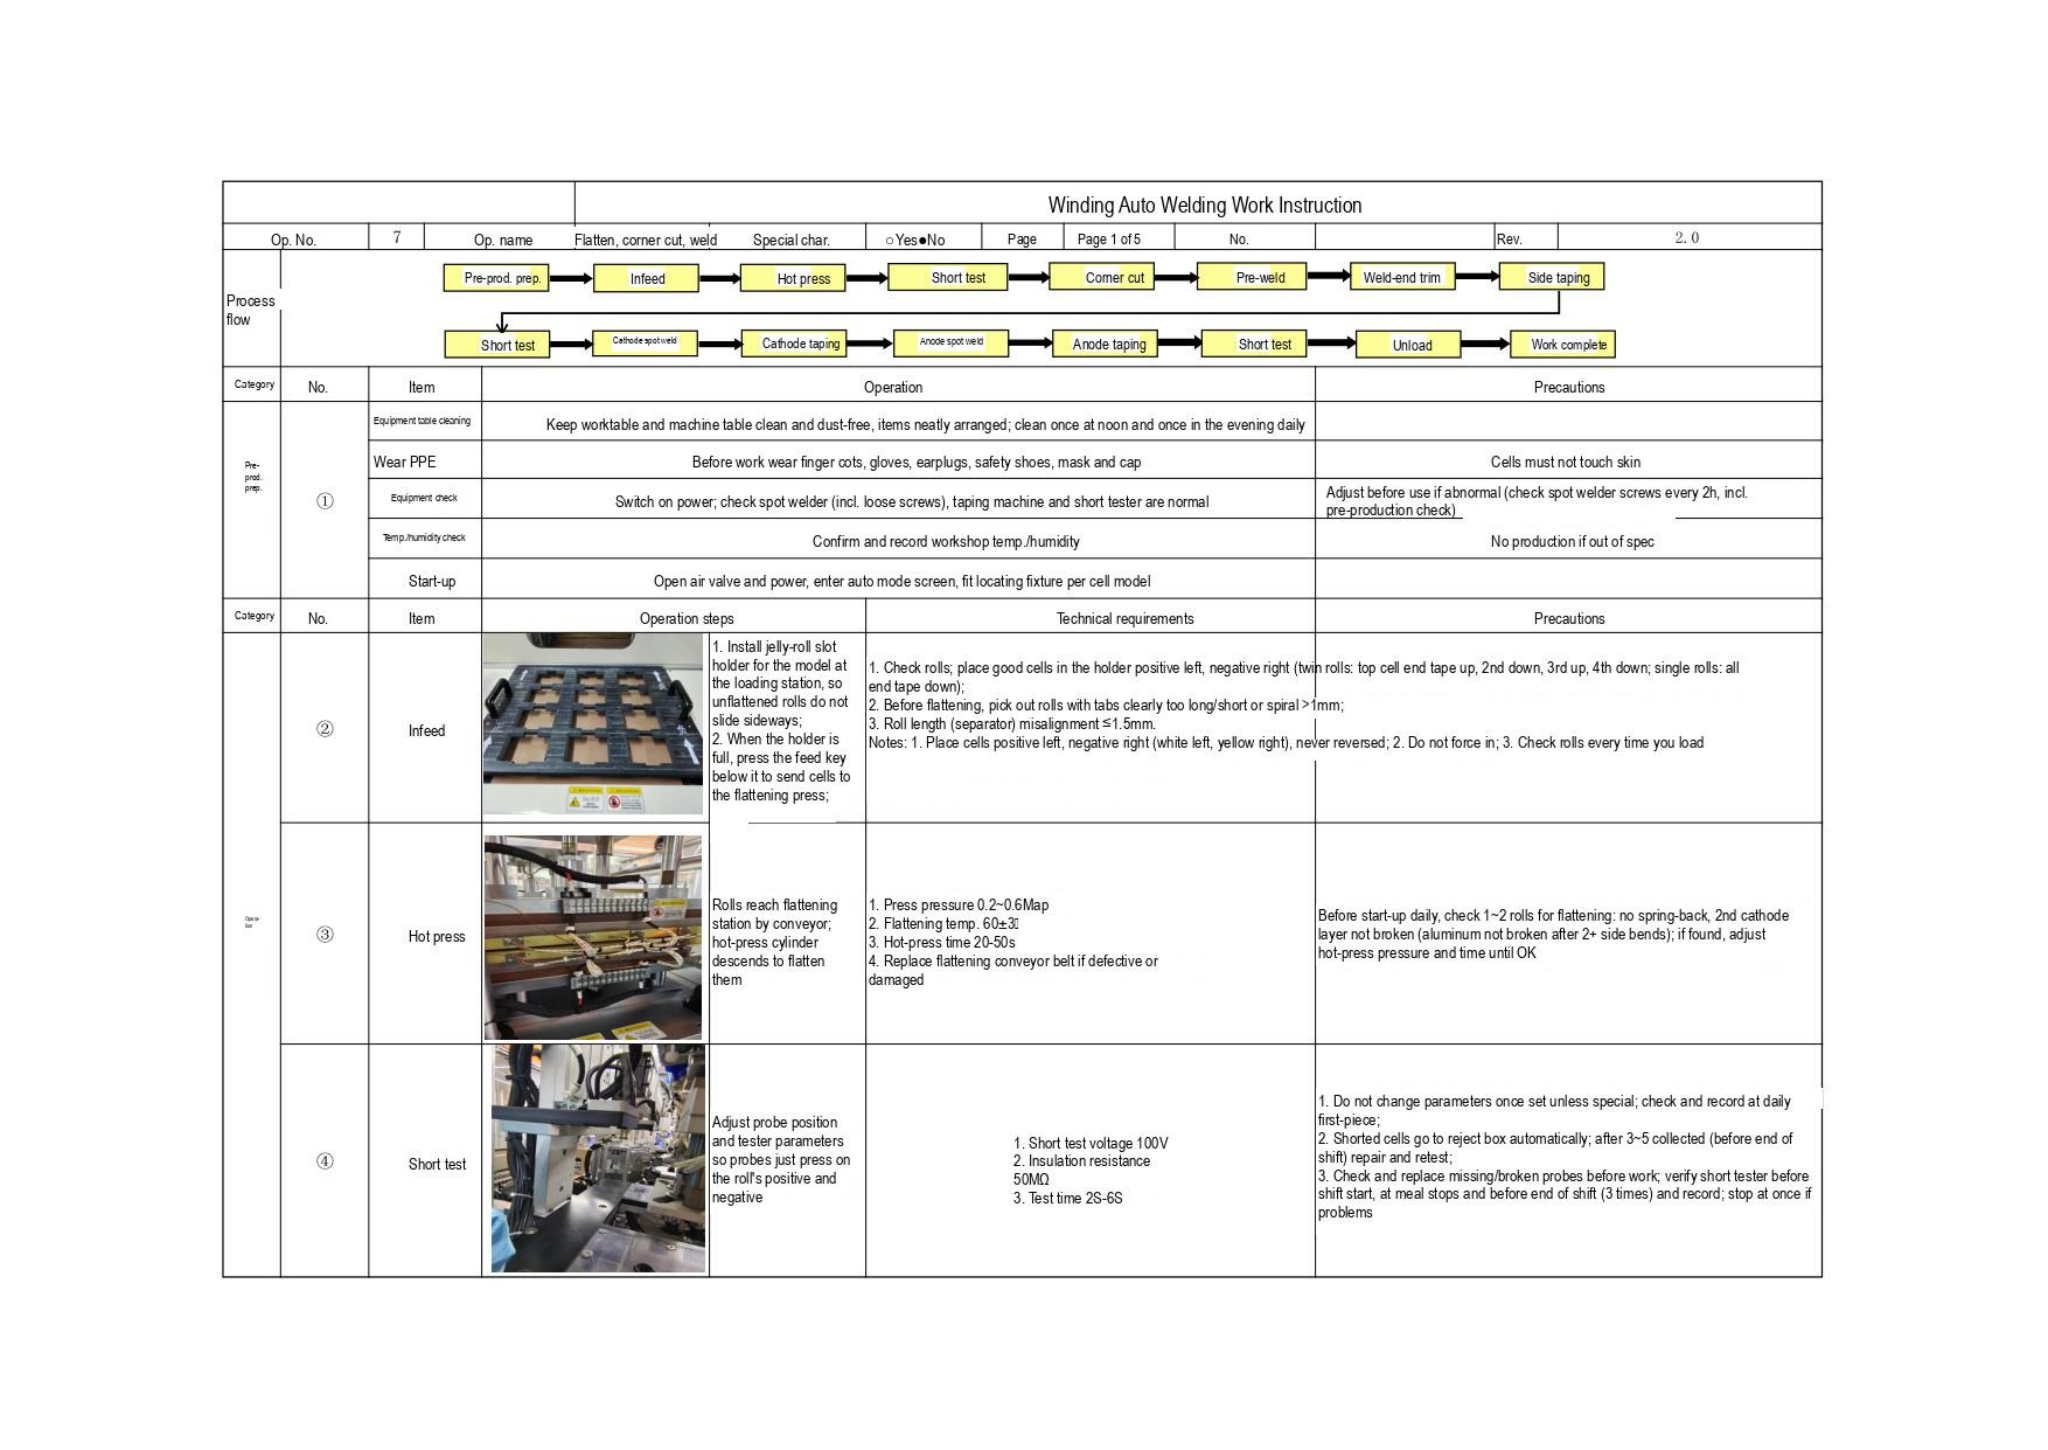Winding Auto Welding Work Instruction

| Op. No. | 7 | Op. name | Flatten, corner cut, weld | Special char. | ○Yes●No | Page | Page 1 of 5 | No. | | Rev. | 2.0 |
|---|---|---|---|---|---|---|---|---|---|---|---|

Process flow

Pre-prod. prep. → Infeed → Hot press → Short test → Corner cut → Pre-weld → Weld-end trim → Side taping → Short test → Cathode spot weld → Cathode taping → Anode spot weld → Anode taping → Short test → Unload → Work complete

| Category | No. | Item | Operation | Precautions |
|---|---|---|---|---|
| Pre-prod. prep. | ① | Equipment table cleaning | Keep worktable and machine table clean and dust-free, items neatly arranged; clean once at noon and once in the evening daily | |
| | | Wear PPE | Before work wear finger cots, gloves, earplugs, safety shoes, mask and cap | Cells must not touch skin |
| | | Equipment check | Switch on power; check spot welder (incl. loose screws), taping machine and short tester are normal | Adjust before use if abnormal (check spot welder screws every 2h, incl. pre-production check) |
| | | Temp./humidity check | Confirm and record workshop temp./humidity | No production if out of spec |
| | | Start-up | Open air valve and power, enter auto mode screen, fit locating fixture per cell model | |

| Category | No. | Item | Operation steps | Technical requirements | Precautions |
|---|---|---|---|---|---|
| | ② | Infeed | 1. Install jelly-roll slot holder for the model at the loading station, so unflattened rolls do not slide sideways;<br>2. When the holder is full, press the feed key below it to send cells to the flattening press; | 1. Check rolls; place good cells in the holder positive left, negative right (twin rolls: top cell end tape up, 2nd down, 3rd up, 4th down; single rolls: all end tape down);<br>2. Before flattening, pick out rolls with tabs clearly too long/short or spiral >1mm;<br>3. Roll length (separator) misalignment ≤1.5mm.<br>Notes: 1. Place cells positive left, negative right (white left, yellow right), never reversed; 2. Do not force in; 3. Check rolls every time you load | |
| | ③ | Hot press | Rolls reach flattening station by conveyor; hot-press cylinder descends to flatten them | 1. Press pressure 0.2~0.6Map<br>2. Flattening temp. 60±3<br>3. Hot-press time 20-50s<br>4. Replace flattening conveyor belt if defective or damaged | Before start-up daily, check 1~2 rolls for flattening: no spring-back, 2nd cathode layer not broken (aluminum not broken after 2+ side bends); if found, adjust hot-press pressure and time until OK |
| | ④ | Short test | Adjust probe position and tester parameters so probes just press on the roll's positive and negative | 1. Short test voltage 100V<br>2. Insulation resistance 50MΩ<br>3. Test time 2S-6S | 1. Do not change parameters once set unless special; check and record at daily first-piece;<br>2. Shorted cells go to reject box automatically; after 3~5 collected (before end of shift) repair and retest;<br>3. Check and replace missing/broken probes before work; verify short tester before shift start, at meal stops and before end of shift (3 times) and record; stop at once if problems |
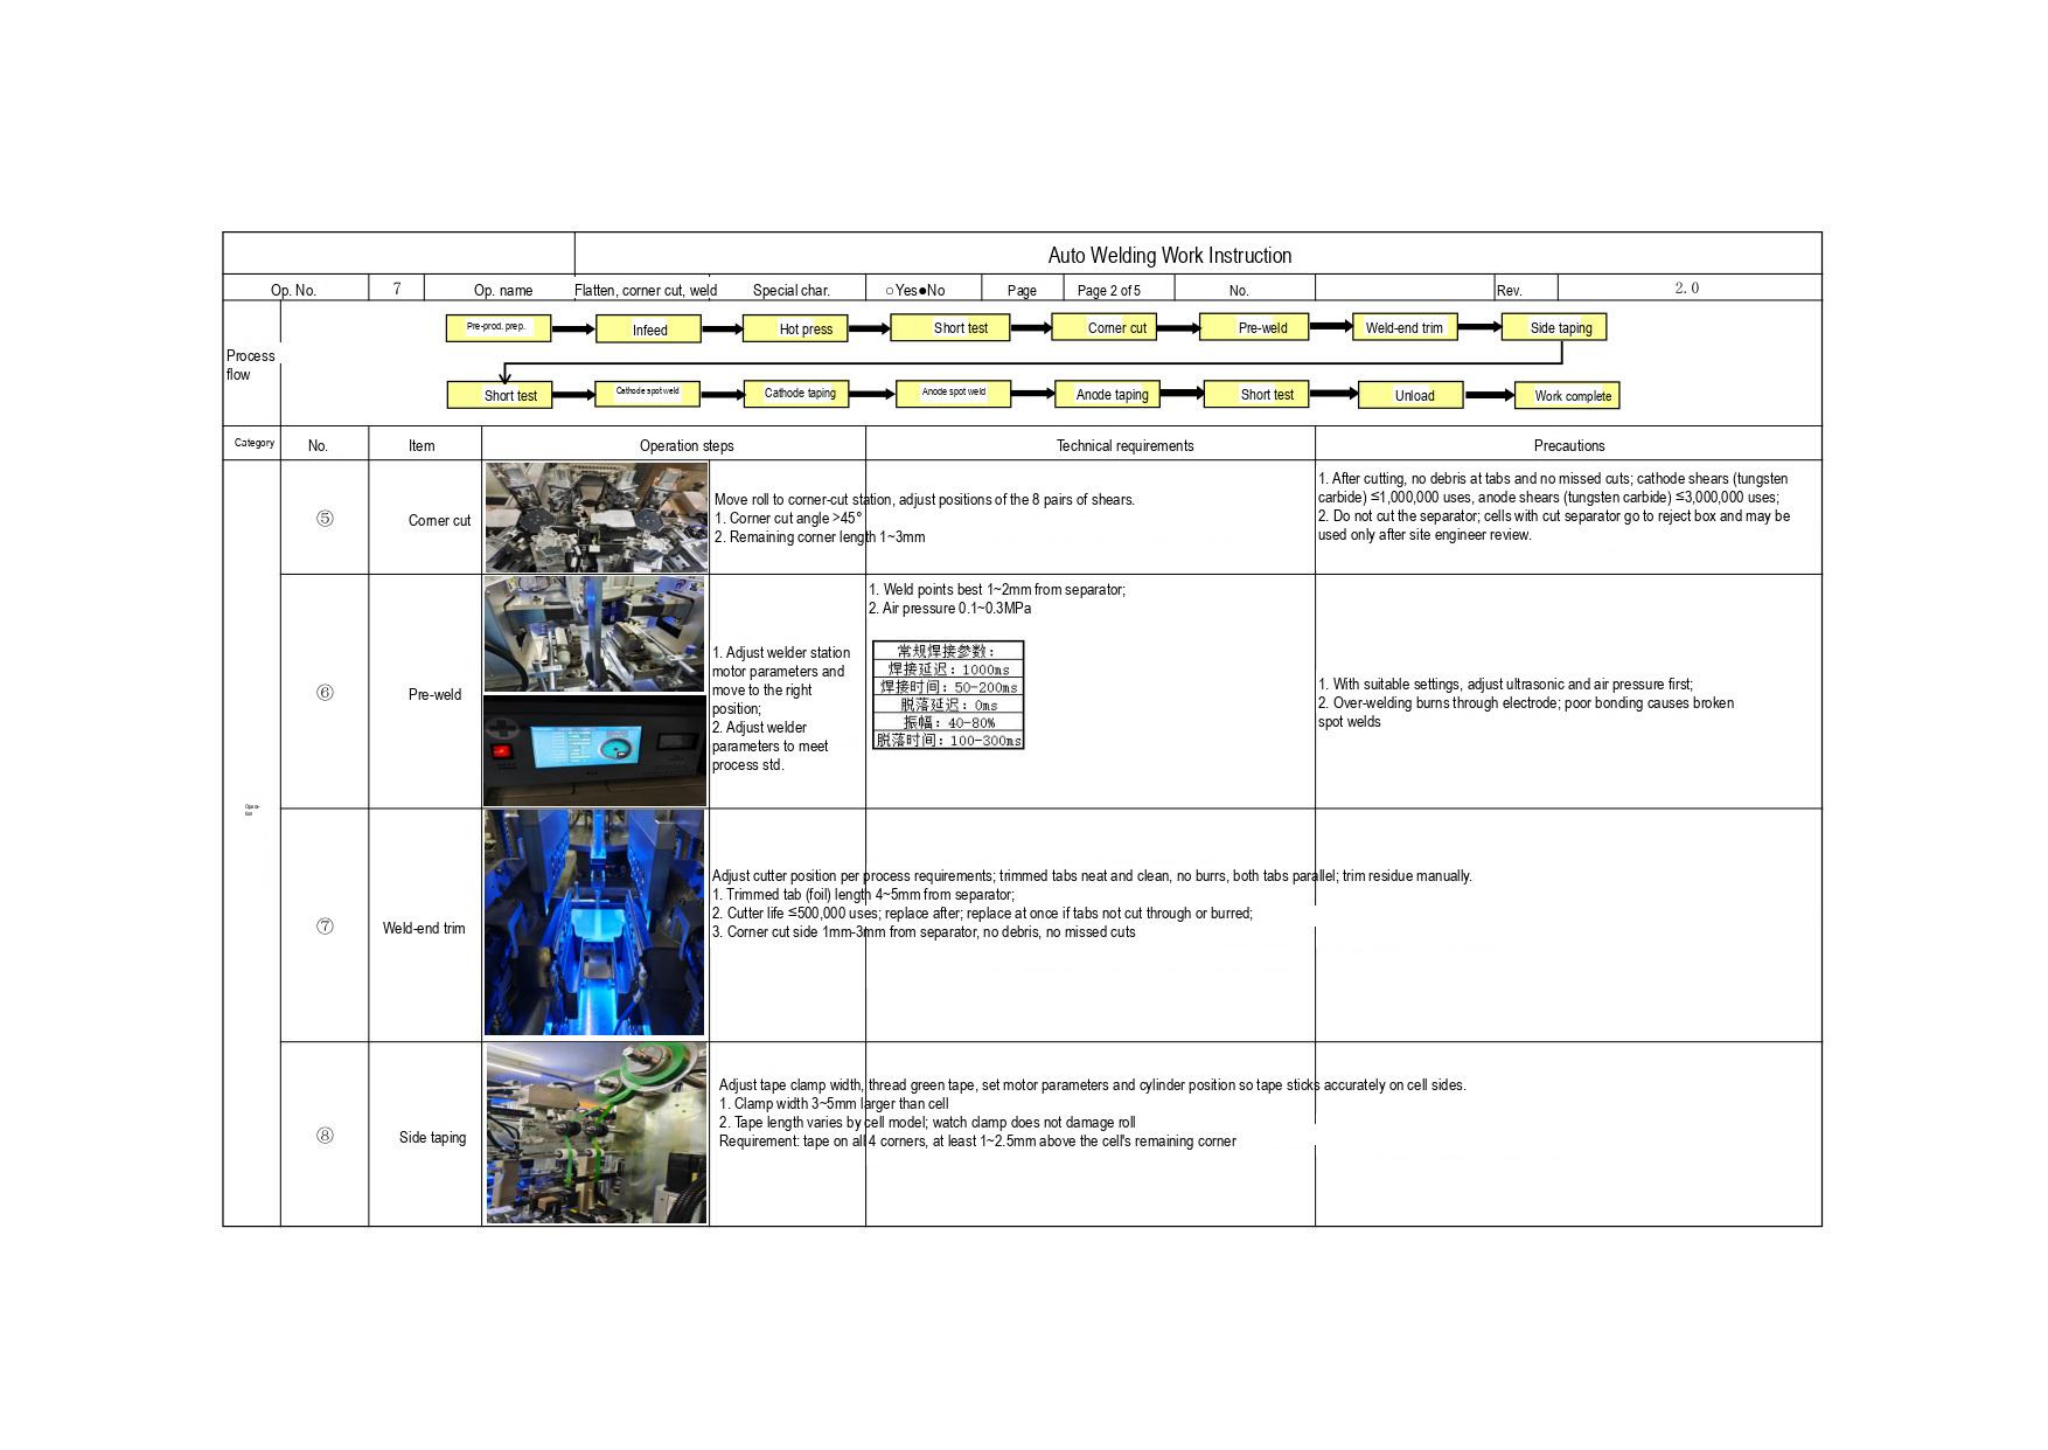Auto Welding Work Instruction

| Op. No. | 7 | Op. name | Flatten, corner cut, weld | Special char. | ○Yes●No | Page | Page 2 of 5 | No. | | Rev. | 2.0 |
|---|---|---|---|---|---|---|---|---|---|---|---|

Process flow

Pre-prod. prep. → Infeed → Hot press → Short test → Corner cut → Pre-weld → Weld-end trim → Side taping → Short test → Cathode spot weld → Cathode taping → Anode spot weld → Anode taping → Short test → Unload → Work complete

| Category | No. | Item | Operation steps | Technical requirements | Precautions |
|---|---|---|---|---|---|
| | ⑤ | Corner cut | Move roll to corner-cut station, adjust positions of the 8 pairs of shears.<br>1. Corner cut angle >45°<br>2. Remaining corner length 1~3mm | | 1. After cutting, no debris at tabs and no missed cuts; cathode shears (tungsten carbide) ≤1,000,000 uses, anode shears (tungsten carbide) ≤3,000,000 uses;<br>2. Do not cut the separator; cells with cut separator go to reject box and may be used only after site engineer review. |
| | ⑥ | Pre-weld | 1. Adjust welder station motor parameters and move to the right position;<br>2. Adjust welder parameters to meet process std. | 1. Weld points best 1~2mm from separator;<br>2. Air pressure 0.1~0.3MPa<br>常规焊接参数:<br>焊接延迟: 1000ms<br>焊接时间: 50-200ms<br>脱落延迟: 0ms<br>振幅: 40-80%<br>脱落时间: 100-300ms | 1. With suitable settings, adjust ultrasonic and air pressure first;<br>2. Over-welding burns through electrode; poor bonding causes broken spot welds |
| | ⑦ | Weld-end trim | Adjust cutter position per process requirements; trimmed tabs neat and clean, no burrs, both tabs parallel; trim residue manually.<br>1. Trimmed tab (foil) length 4~5mm from separator;<br>2. Cutter life ≤500,000 uses; replace after; replace at once if tabs not cut through or burred;<br>3. Corner cut side 1mm-3mm from separator, no debris, no missed cuts | | |
| | ⑧ | Side taping | Adjust tape clamp width, thread green tape, set motor parameters and cylinder position so tape sticks accurately on cell sides.<br>1. Clamp width 3~5mm larger than cell<br>2. Tape length varies by cell model; watch clamp does not damage roll<br>Requirement: tape on all 4 corners, at least 1~2.5mm above the cell's remaining corner | | |
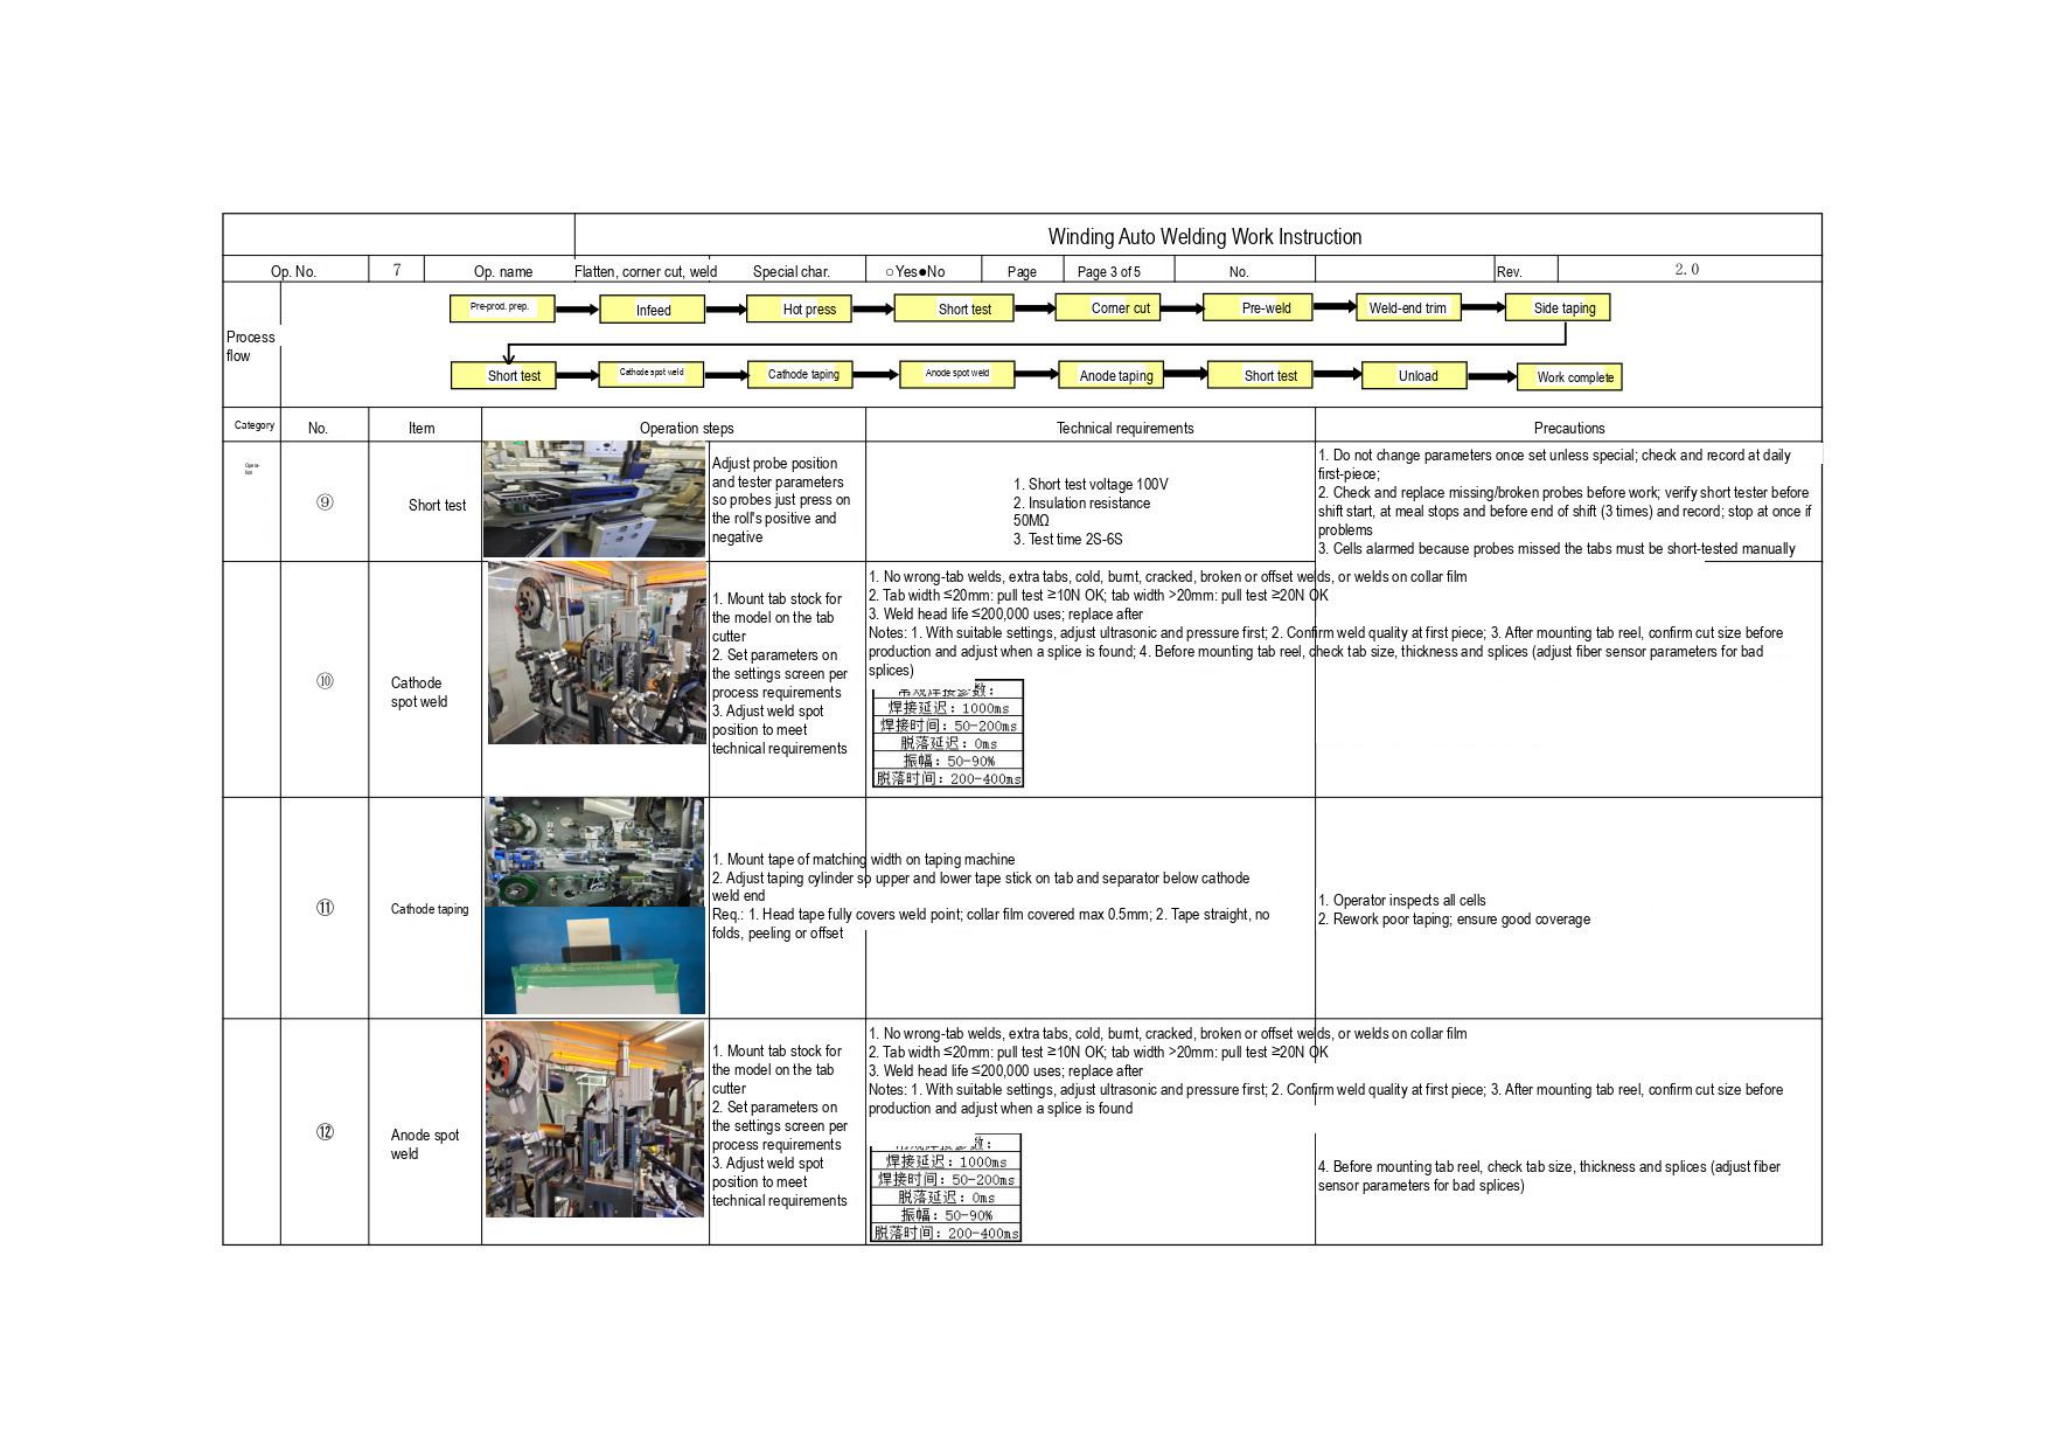**Winding Auto Welding Work Instruction**

| Op. No. | 7 | Op. name | Flatten, corner cut, weld | Special char. | ○Yes●No | Page | Page 3 of 5 | No. | | Rev. | 2. 0 |
|---|---|---|---|---|---|---|---|---|---|---|---|

Process flow

Pre-prod. prep. → Infeed → Hot press → Short test → Corner cut → Pre-weld → Weld-end trim → Side taping → Short test → Cathode spot weld → Cathode taping → Anode spot weld → Anode taping → Short test → Unload → Work complete

| Category | No. | Item | Operation steps | Technical requirements | Precautions |
|---|---|---|---|---|---|
| | ⑨ | Short test | Adjust probe position and tester parameters so probes just press on the roll's positive and negative | 1. Short test voltage 100V<br>2. Insulation resistance 50MΩ<br>3. Test time 2S-6S | 1. Do not change parameters once set unless special; check and record at daily first-piece;<br>2. Check and replace missing/broken probes before work; verify short tester before shift start, at meal stops and before end of shift (3 times) and record; stop at once if problems<br>3. Cells alarmed because probes missed the tabs must be short-tested manually |
| | ⑩ | Cathode spot weld | 1. Mount tab stock for the model on the tab cutter<br>2. Set parameters on the settings screen per process requirements<br>3. Adjust weld spot position to meet technical requirements | 1. No wrong-tab welds, extra tabs, cold, burnt, cracked, broken or offset welds, or welds on collar film<br>2. Tab width ≤20mm: pull test ≥10N OK; tab width >20mm: pull test ≥20N OK<br>3. Weld head life ≤200,000 uses; replace after<br>Notes: 1. With suitable settings, adjust ultrasonic and pressure first; 2. Confirm weld quality at first piece; 3. After mounting tab reel, confirm cut size before production and adjust when a splice is found; 4. Before mounting tab reel, check tab size, thickness and splices (adjust fiber sensor parameters for bad splices)<br>焊接延迟：1000ms<br>焊接时间：50-200ms<br>脱落延迟：0ms<br>振幅：50-90%<br>脱落时间：200-400ms | |
| | ⑪ | Cathode taping | 1. Mount tape of matching width on taping machine<br>2. Adjust taping cylinder so upper and lower tape stick on tab and separator below cathode weld end<br>Req.: 1. Head tape fully covers weld point; collar film covered max 0.5mm; 2. Tape straight, no folds, peeling or offset | | 1. Operator inspects all cells<br>2. Rework poor taping; ensure good coverage |
| | ⑫ | Anode spot weld | 1. Mount tab stock for the model on the tab cutter<br>2. Set parameters on the settings screen per process requirements<br>3. Adjust weld spot position to meet technical requirements | 1. No wrong-tab welds, extra tabs, cold, burnt, cracked, broken or offset welds, or welds on collar film<br>2. Tab width ≤20mm: pull test ≥10N OK; tab width >20mm: pull test ≥20N OK<br>3. Weld head life ≤200,000 uses; replace after<br>Notes: 1. With suitable settings, adjust ultrasonic and pressure first; 2. Confirm weld quality at first piece; 3. After mounting tab reel, confirm cut size before production and adjust when a splice is found<br>焊接延迟：1000ms<br>焊接时间：50-200ms<br>脱落延迟：0ms<br>振幅：50-90%<br>脱落时间：200-400ms | 4. Before mounting tab reel, check tab size, thickness and splices (adjust fiber sensor parameters for bad splices) |
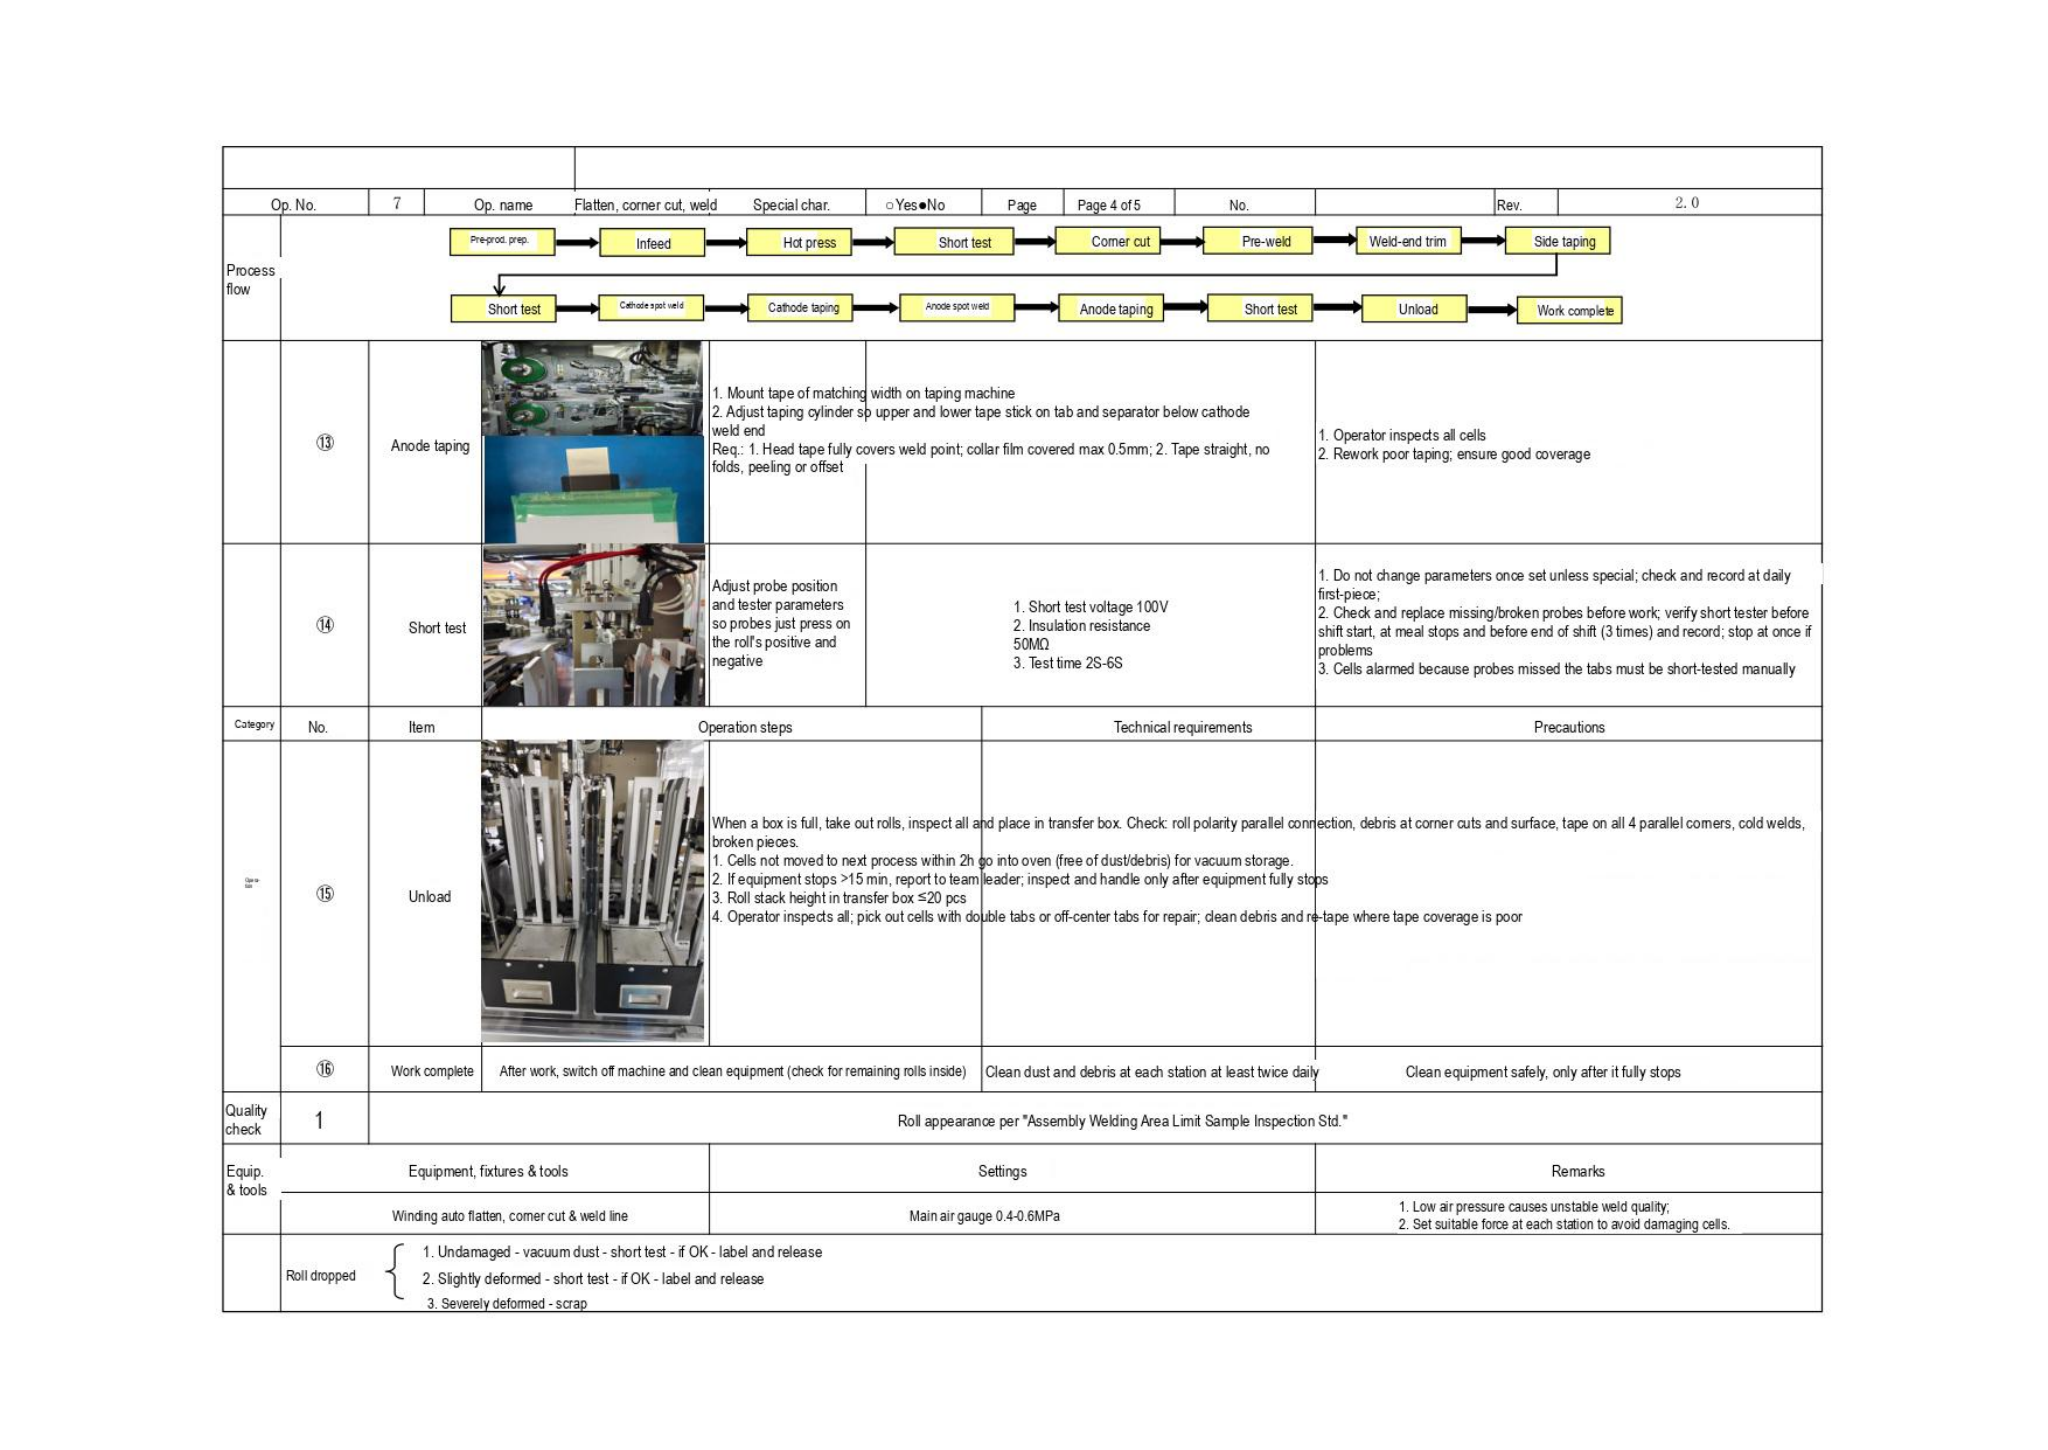| Op. No. | 7 | Op. name | Flatten, corner cut, weld | Special char. | ○Yes●No | Page | Page 4 of 5 | No. | | Rev. | 2.0 |
|---|---|---|---|---|---|---|---|---|---|---|---|

| Process flow | Pre-prod. prep. → Infeed → Hot press → Short test → Corner cut → Pre-weld → Weld-end trim → Side taping → Short test → Cathode spot weld → Cathode taping → Anode spot weld → Anode taping → Short test → Unload → Work complete |
|---|---|

| Category | No. | Item | Operation steps | Technical requirements | Precautions |
|---|---|---|---|---|---|
| | ⑬ | Anode taping | 1. Mount tape of matching width on taping machine<br>2. Adjust taping cylinder so upper and lower tape stick on tab and separator below cathode weld end<br>Req.: 1. Head tape fully covers weld point; collar film covered max 0.5mm; 2. Tape straight, no folds, peeling or offset | | 1. Operator inspects all cells<br>2. Rework poor taping; ensure good coverage |
| | ⑭ | Short test | Adjust probe position and tester parameters so probes just press on the roll's positive and negative | 1. Short test voltage 100V<br>2. Insulation resistance 50MΩ<br>3. Test time 2S-6S | 1. Do not change parameters once set unless special; check and record at daily first-piece;<br>2. Check and replace missing/broken probes before work; verify short tester before shift start, at meal stops and before end of shift (3 times) and record; stop at once if problems<br>3. Cells alarmed because probes missed the tabs must be short-tested manually |
| | ⑮ | Unload | When a box is full, take out rolls, inspect all and place in transfer box. Check: roll polarity parallel connection, debris at corner cuts and surface, tape on all 4 parallel corners, cold welds, broken pieces.<br>1. Cells not moved to next process within 2h go into oven (free of dust/debris) for vacuum storage.<br>2. If equipment stops >15 min, report to team leader; inspect and handle only after equipment fully stops<br>3. Roll stack height in transfer box ≤20 pcs<br>4. Operator inspects all; pick out cells with double tabs or off-center tabs for repair; clean debris and re-tape where tape coverage is poor | | |
| | ⑯ | Work complete | After work, switch off machine and clean equipment (check for remaining rolls inside) | Clean dust and debris at each station at least twice daily | Clean equipment safely, only after it fully stops |

| Quality check | 1 | Roll appearance per "Assembly Welding Area Limit Sample Inspection Std." |
|---|---|---|

| Equip. & tools | Equipment, fixtures & tools | Settings | Remarks |
|---|---|---|---|
| | Winding auto flatten, corner cut & weld line | Main air gauge 0.4-0.6MPa | 1. Low air pressure causes unstable weld quality;<br>2. Set suitable force at each station to avoid damaging cells. |

Roll dropped
1. Undamaged - vacuum dust - short test - if OK - label and release
2. Slightly deformed - short test - if OK - label and release
3. Severely deformed - scrap
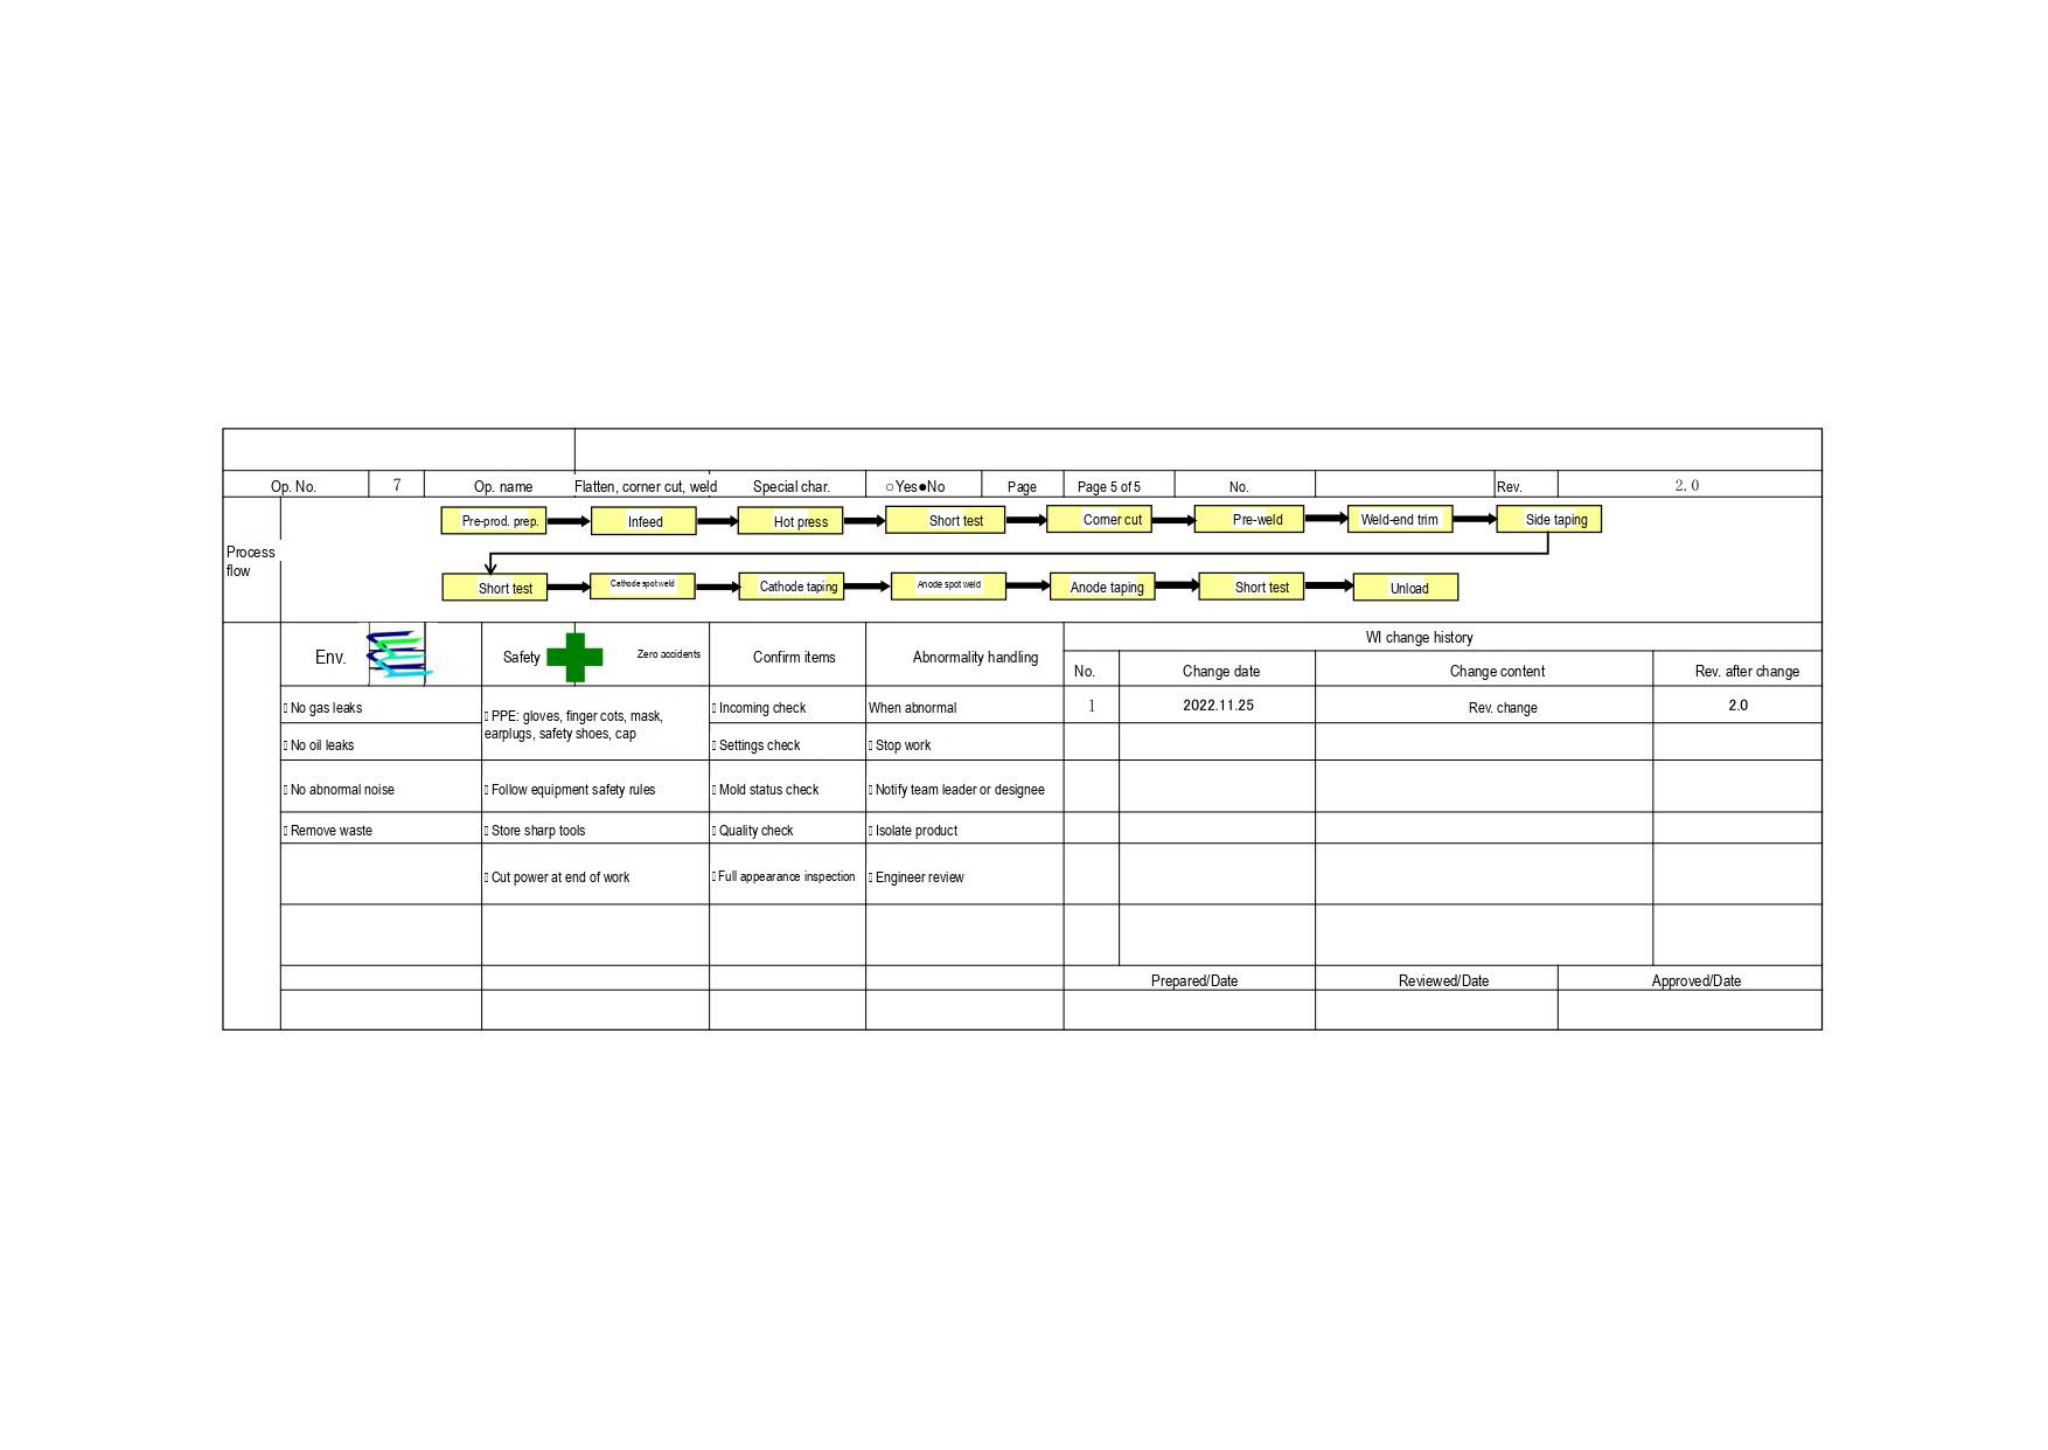| Op. No. | 7 | Op. name | Flatten, corner cut, weld | Special char. | ○Yes●No | Page | Page 5 of 5 | No. | | Rev. | 2.0 |
|---|---|---|---|---|---|---|---|---|---|---|---|

Process flow

Pre-prod. prep. → Infeed → Hot press → Short test → Corner cut → Pre-weld → Weld-end trim → Side taping → Short test → Cathode spot weld → Cathode taping → Anode spot weld → Anode taping → Short test → Unload

| Env. | Safety Zero accidents | Confirm items | Abnormality handling |
|---|---|---|---|
| No gas leaks | PPE: gloves, finger cots, mask, earplugs, safety shoes, cap | Incoming check | When abnormal |
| No oil leaks | | Settings check | Stop work |
| No abnormal noise | Follow equipment safety rules | Mold status check | Notify team leader or designee |
| Remove waste | Store sharp tools | Quality check | Isolate product |
| | Cut power at end of work | Full appearance inspection | Engineer review |

WI change history

| No. | Change date | Change content | Rev. after change |
|---|---|---|---|
| 1 | 2022.11.25 | Rev. change | 2.0 |
| | | | |
| | | | |
| | | | |
| | | | |
| | | | |

| Prepared/Date | Reviewed/Date | Approved/Date |
|---|---|---|
| | | |